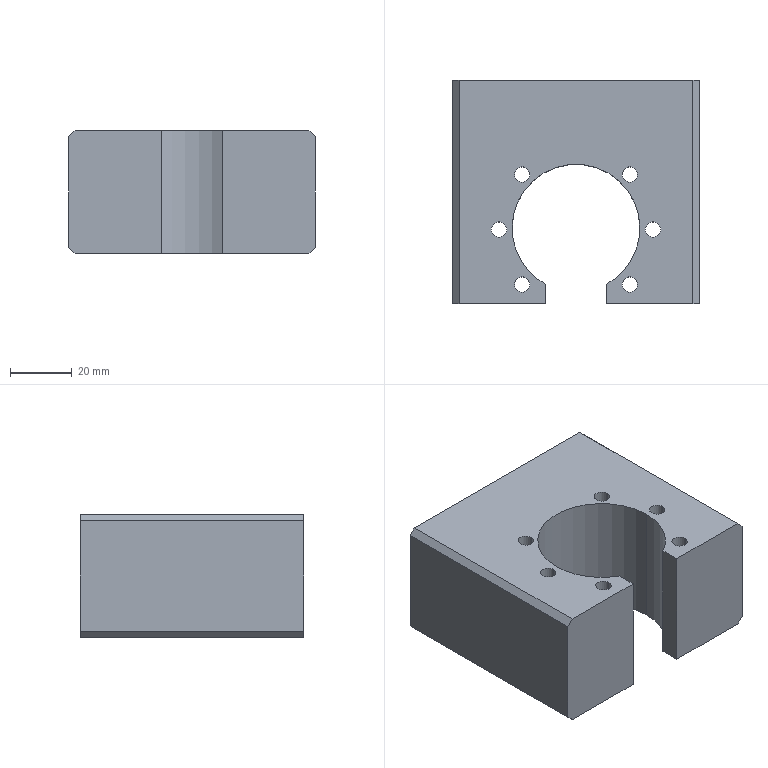Part | SolidWorks | features HoleWzd 2, Chamfer 1, Extrusion 1, ICE 1 | 1 solid | 52 faces | box 80 x 72.5 x 40 mm | volume 167108 mm3 | cylinder 27 | plane 13 | cone 12 | commonest cylinder face diameters 5 x24 41.5 x3
STEP:
#1=CARTESIAN_POINT('',(-27.5,21.25,-13.5));
#2=VERTEX_POINT('',#1);
#3=CARTESIAN_POINT('',(-27.5,21.25,-8.5));
#4=VERTEX_POINT('',#3);
#5=CARTESIAN_POINT('',(-27.5,21.25,-11.));
#6=DIRECTION('',(0.,1.,0.));
#7=DIRECTION('',(0.,0.,1.));
#8=AXIS2_PLACEMENT_3D('',#5,#6,#7);
#9=CIRCLE('',#8,2.5);
#10=EDGE_CURVE('',#2,#4,#9,.T.);
#11=ORIENTED_EDGE('',*,*,#10,.F.);
#12=CARTESIAN_POINT('',(-27.5,36.25,-13.5));
#13=VERTEX_POINT('',#12);
#14=CARTESIAN_POINT('',(-27.5,36.25,-13.5));
#15=DIRECTION('',(0.,1.,0.));
#16=VECTOR('',#15,1000.);
#17=LINE('',#14,#16);
#18=EDGE_CURVE('',#2,#13,#17,.T.);
#19=ORIENTED_EDGE('',*,*,#18,.T.);
#20=CARTESIAN_POINT('',(-27.5,36.25,-8.5));
#21=VERTEX_POINT('',#20);
#22=CARTESIAN_POINT('',(-27.5,36.25,-11.));
#23=DIRECTION('',(0.,1.,0.));
#24=DIRECTION('',(0.,0.,1.));
#25=AXIS2_PLACEMENT_3D('',#22,#23,#24);
#26=CIRCLE('',#25,2.5);
#27=EDGE_CURVE('',#13,#21,#26,.T.);
#28=ORIENTED_EDGE('',*,*,#27,.T.);
#29=CARTESIAN_POINT('',(-27.5,36.25,-8.5));
#30=DIRECTION('',(0.,1.,0.));
#31=VECTOR('',#30,1000.);
#32=LINE('',#29,#31);
#33=EDGE_CURVE('',#4,#21,#32,.T.);
#34=ORIENTED_EDGE('',*,*,#33,.F.);
#35=EDGE_LOOP('',(#11,#19,#28,#34));
#36=FACE_OUTER_BOUND('',#35,.T.);
#37=CARTESIAN_POINT('',(-27.5,36.25,-11.));
#38=DIRECTION('',(0.,1.,0.));
#39=DIRECTION('',(0.,0.,1.));
#40=AXIS2_PLACEMENT_3D('',#37,#38,#39);
#41=CYLINDRICAL_SURFACE('',#40,2.5);
#42=ADVANCED_FACE('',(#36),#41,.F.);
#43=CARTESIAN_POINT('',(-27.5,19.748,-11.));
#44=VERTEX_POINT('',#43);
#45=CARTESIAN_POINT('',(-27.5,21.25,-8.5));
#46=DIRECTION('',(0.,0.515,0.8572));
#47=VECTOR('',#46,1000.);
#48=LINE('',#45,#47);
#49=EDGE_CURVE('',#44,#4,#48,.T.);
#50=ORIENTED_EDGE('',*,*,#49,.F.);
#51=CARTESIAN_POINT('',(-27.5,21.25,-13.5));
#52=DIRECTION('',(0.,0.515,-0.8572));
#53=VECTOR('',#52,1000.);
#54=LINE('',#51,#53);
#55=EDGE_CURVE('',#44,#2,#54,.T.);
#56=ORIENTED_EDGE('',*,*,#55,.T.);
#57=ORIENTED_EDGE('',*,*,#10,.T.);
#58=EDGE_LOOP('',(#50,#56,#57));
#59=FACE_OUTER_BOUND('',#58,.T.);
#60=CARTESIAN_POINT('',(-27.5,21.25,-11.));
#61=DIRECTION('',(0.,1.,0.));
#62=DIRECTION('',(0.,0.,1.));
#63=AXIS2_PLACEMENT_3D('',#60,#61,#62);
#64=CONICAL_SURFACE('',#63,2.5,1.03);
#65=ADVANCED_FACE('',(#59),#64,.F.);
#66=CARTESIAN_POINT('',(-27.5,21.25,8.5));
#67=VERTEX_POINT('',#66);
#68=CARTESIAN_POINT('',(-27.5,21.25,13.5));
#69=VERTEX_POINT('',#68);
#70=CARTESIAN_POINT('',(-27.5,21.25,11.));
#71=DIRECTION('',(0.,1.,0.));
#72=DIRECTION('',(0.,0.,1.));
#73=AXIS2_PLACEMENT_3D('',#70,#71,#72);
#74=CIRCLE('',#73,2.5);
#75=EDGE_CURVE('',#67,#69,#74,.T.);
#76=ORIENTED_EDGE('',*,*,#75,.F.);
#77=CARTESIAN_POINT('',(-27.5,36.25,8.5));
#78=VERTEX_POINT('',#77);
#79=CARTESIAN_POINT('',(-27.5,36.25,8.5));
#80=DIRECTION('',(0.,1.,0.));
#81=VECTOR('',#80,1000.);
#82=LINE('',#79,#81);
#83=EDGE_CURVE('',#67,#78,#82,.T.);
#84=ORIENTED_EDGE('',*,*,#83,.T.);
#85=CARTESIAN_POINT('',(-27.5,36.25,13.5));
#86=VERTEX_POINT('',#85);
#87=CARTESIAN_POINT('',(-27.5,36.25,11.));
#88=DIRECTION('',(0.,1.,0.));
#89=DIRECTION('',(0.,0.,1.));
#90=AXIS2_PLACEMENT_3D('',#87,#88,#89);
#91=CIRCLE('',#90,2.5);
#92=EDGE_CURVE('',#78,#86,#91,.T.);
#93=ORIENTED_EDGE('',*,*,#92,.T.);
#94=CARTESIAN_POINT('',(-27.5,36.25,13.5));
#95=DIRECTION('',(0.,1.,0.));
#96=VECTOR('',#95,1000.);
#97=LINE('',#94,#96);
#98=EDGE_CURVE('',#69,#86,#97,.T.);
#99=ORIENTED_EDGE('',*,*,#98,.F.);
#100=EDGE_LOOP('',(#76,#84,#93,#99));
#101=FACE_OUTER_BOUND('',#100,.T.);
#102=CARTESIAN_POINT('',(-27.5,36.25,11.));
#103=DIRECTION('',(0.,1.,0.));
#104=DIRECTION('',(0.,0.,1.));
#105=AXIS2_PLACEMENT_3D('',#102,#103,#104);
#106=CYLINDRICAL_SURFACE('',#105,2.5);
#107=ADVANCED_FACE('',(#101),#106,.F.);
#108=CARTESIAN_POINT('',(-27.5,19.748,11.));
#109=VERTEX_POINT('',#108);
#110=CARTESIAN_POINT('',(-27.5,21.25,13.5));
#111=DIRECTION('',(0.,0.515,0.8572));
#112=VECTOR('',#111,1000.);
#113=LINE('',#110,#112);
#114=EDGE_CURVE('',#109,#69,#113,.T.);
#115=ORIENTED_EDGE('',*,*,#114,.F.);
#116=CARTESIAN_POINT('',(-27.5,21.25,8.5));
#117=DIRECTION('',(0.,0.515,-0.8572));
#118=VECTOR('',#117,1000.);
#119=LINE('',#116,#118);
#120=EDGE_CURVE('',#109,#67,#119,.T.);
#121=ORIENTED_EDGE('',*,*,#120,.T.);
#122=ORIENTED_EDGE('',*,*,#75,.T.);
#123=EDGE_LOOP('',(#115,#121,#122));
#124=FACE_OUTER_BOUND('',#123,.T.);
#125=CARTESIAN_POINT('',(-27.5,21.25,11.));
#126=DIRECTION('',(0.,1.,0.));
#127=DIRECTION('',(0.,0.,1.));
#128=AXIS2_PLACEMENT_3D('',#125,#126,#127);
#129=CONICAL_SURFACE('',#128,2.5,1.03);
#130=ADVANCED_FACE('',(#124),#129,.F.);
#131=CARTESIAN_POINT('',(27.5,21.25,8.5));
#132=VERTEX_POINT('',#131);
#133=CARTESIAN_POINT('',(27.5,21.25,13.5));
#134=VERTEX_POINT('',#133);
#135=CARTESIAN_POINT('',(27.5,21.25,11.));
#136=DIRECTION('',(0.,1.,0.));
#137=DIRECTION('',(0.,0.,1.));
#138=AXIS2_PLACEMENT_3D('',#135,#136,#137);
#139=CIRCLE('',#138,2.5);
#140=EDGE_CURVE('',#132,#134,#139,.T.);
#141=ORIENTED_EDGE('',*,*,#140,.F.);
#142=CARTESIAN_POINT('',(27.5,36.25,8.5));
#143=VERTEX_POINT('',#142);
#144=CARTESIAN_POINT('',(27.5,36.25,8.5));
#145=DIRECTION('',(0.,1.,0.));
#146=VECTOR('',#145,1000.);
#147=LINE('',#144,#146);
#148=EDGE_CURVE('',#132,#143,#147,.T.);
#149=ORIENTED_EDGE('',*,*,#148,.T.);
#150=CARTESIAN_POINT('',(27.5,36.25,13.5));
#151=VERTEX_POINT('',#150);
#152=CARTESIAN_POINT('',(27.5,36.25,11.));
#153=DIRECTION('',(0.,1.,0.));
#154=DIRECTION('',(0.,0.,1.));
#155=AXIS2_PLACEMENT_3D('',#152,#153,#154);
#156=CIRCLE('',#155,2.5);
#157=EDGE_CURVE('',#143,#151,#156,.T.);
#158=ORIENTED_EDGE('',*,*,#157,.T.);
#159=CARTESIAN_POINT('',(27.5,36.25,13.5));
#160=DIRECTION('',(0.,1.,0.));
#161=VECTOR('',#160,1000.);
#162=LINE('',#159,#161);
#163=EDGE_CURVE('',#134,#151,#162,.T.);
#164=ORIENTED_EDGE('',*,*,#163,.F.);
#165=EDGE_LOOP('',(#141,#149,#158,#164));
#166=FACE_OUTER_BOUND('',#165,.T.);
#167=CARTESIAN_POINT('',(27.5,36.25,11.));
#168=DIRECTION('',(0.,1.,0.));
#169=DIRECTION('',(0.,0.,1.));
#170=AXIS2_PLACEMENT_3D('',#167,#168,#169);
#171=CYLINDRICAL_SURFACE('',#170,2.5);
#172=ADVANCED_FACE('',(#166),#171,.F.);
#173=CARTESIAN_POINT('',(27.5,19.748,11.));
#174=VERTEX_POINT('',#173);
#175=CARTESIAN_POINT('',(27.5,21.25,13.5));
#176=DIRECTION('',(0.,0.515,0.8572));
#177=VECTOR('',#176,1000.);
#178=LINE('',#175,#177);
#179=EDGE_CURVE('',#174,#134,#178,.T.);
#180=ORIENTED_EDGE('',*,*,#179,.F.);
#181=CARTESIAN_POINT('',(27.5,21.25,8.5));
#182=DIRECTION('',(0.,0.515,-0.8572));
#183=VECTOR('',#182,1000.);
#184=LINE('',#181,#183);
#185=EDGE_CURVE('',#174,#132,#184,.T.);
#186=ORIENTED_EDGE('',*,*,#185,.T.);
#187=ORIENTED_EDGE('',*,*,#140,.T.);
#188=EDGE_LOOP('',(#180,#186,#187));
#189=FACE_OUTER_BOUND('',#188,.T.);
#190=CARTESIAN_POINT('',(27.5,21.25,11.));
#191=DIRECTION('',(0.,1.,0.));
#192=DIRECTION('',(0.,0.,1.));
#193=AXIS2_PLACEMENT_3D('',#190,#191,#192);
#194=CONICAL_SURFACE('',#193,2.5,1.03);
#195=ADVANCED_FACE('',(#189),#194,.F.);
#196=CARTESIAN_POINT('',(27.5,21.25,-13.5));
#197=VERTEX_POINT('',#196);
#198=CARTESIAN_POINT('',(27.5,21.25,-8.5));
#199=VERTEX_POINT('',#198);
#200=CARTESIAN_POINT('',(27.5,21.25,-11.));
#201=DIRECTION('',(0.,1.,0.));
#202=DIRECTION('',(0.,0.,1.));
#203=AXIS2_PLACEMENT_3D('',#200,#201,#202);
#204=CIRCLE('',#203,2.5);
#205=EDGE_CURVE('',#197,#199,#204,.T.);
#206=ORIENTED_EDGE('',*,*,#205,.F.);
#207=CARTESIAN_POINT('',(27.5,36.25,-13.5));
#208=VERTEX_POINT('',#207);
#209=CARTESIAN_POINT('',(27.5,36.25,-13.5));
#210=DIRECTION('',(0.,1.,0.));
#211=VECTOR('',#210,1000.);
#212=LINE('',#209,#211);
#213=EDGE_CURVE('',#197,#208,#212,.T.);
#214=ORIENTED_EDGE('',*,*,#213,.T.);
#215=CARTESIAN_POINT('',(27.5,36.25,-8.5));
#216=VERTEX_POINT('',#215);
#217=CARTESIAN_POINT('',(27.5,36.25,-11.));
#218=DIRECTION('',(0.,1.,0.));
#219=DIRECTION('',(0.,0.,1.));
#220=AXIS2_PLACEMENT_3D('',#217,#218,#219);
#221=CIRCLE('',#220,2.5);
#222=EDGE_CURVE('',#208,#216,#221,.T.);
#223=ORIENTED_EDGE('',*,*,#222,.T.);
#224=CARTESIAN_POINT('',(27.5,36.25,-8.5));
#225=DIRECTION('',(0.,1.,0.));
#226=VECTOR('',#225,1000.);
#227=LINE('',#224,#226);
#228=EDGE_CURVE('',#199,#216,#227,.T.);
#229=ORIENTED_EDGE('',*,*,#228,.F.);
#230=EDGE_LOOP('',(#206,#214,#223,#229));
#231=FACE_OUTER_BOUND('',#230,.T.);
#232=CARTESIAN_POINT('',(27.5,36.25,-11.));
#233=DIRECTION('',(0.,1.,0.));
#234=DIRECTION('',(0.,0.,1.));
#235=AXIS2_PLACEMENT_3D('',#232,#233,#234);
#236=CYLINDRICAL_SURFACE('',#235,2.5);
#237=ADVANCED_FACE('',(#231),#236,.F.);
#238=CARTESIAN_POINT('',(27.5,19.748,-11.));
#239=VERTEX_POINT('',#238);
#240=CARTESIAN_POINT('',(27.5,21.25,-8.5));
#241=DIRECTION('',(0.,0.515,0.8572));
#242=VECTOR('',#241,1000.);
#243=LINE('',#240,#242);
#244=EDGE_CURVE('',#239,#199,#243,.T.);
#245=ORIENTED_EDGE('',*,*,#244,.F.);
#246=CARTESIAN_POINT('',(27.5,21.25,-13.5));
#247=DIRECTION('',(0.,0.515,-0.8572));
#248=VECTOR('',#247,1000.);
#249=LINE('',#246,#248);
#250=EDGE_CURVE('',#239,#197,#249,.T.);
#251=ORIENTED_EDGE('',*,*,#250,.T.);
#252=ORIENTED_EDGE('',*,*,#205,.T.);
#253=EDGE_LOOP('',(#245,#251,#252));
#254=FACE_OUTER_BOUND('',#253,.T.);
#255=CARTESIAN_POINT('',(27.5,21.25,-11.));
#256=DIRECTION('',(0.,1.,0.));
#257=DIRECTION('',(0.,0.,1.));
#258=AXIS2_PLACEMENT_3D('',#255,#256,#257);
#259=CONICAL_SURFACE('',#258,2.5,1.03);
#260=ADVANCED_FACE('',(#254),#259,.F.);
#261=CARTESIAN_POINT('',(0.,21.25,-13.5));
#262=VERTEX_POINT('',#261);
#263=CARTESIAN_POINT('',(0.,21.25,-8.5));
#264=VERTEX_POINT('',#263);
#265=CARTESIAN_POINT('',(0.,21.25,-11.));
#266=DIRECTION('',(0.,1.,0.));
#267=DIRECTION('',(0.,0.,1.));
#268=AXIS2_PLACEMENT_3D('',#265,#266,#267);
#269=CIRCLE('',#268,2.5);
#270=EDGE_CURVE('',#262,#264,#269,.T.);
#271=ORIENTED_EDGE('',*,*,#270,.F.);
#272=CARTESIAN_POINT('',(0.,36.25,-13.5));
#273=VERTEX_POINT('',#272);
#274=CARTESIAN_POINT('',(0.,36.25,-13.5));
#275=DIRECTION('',(0.,1.,0.));
#276=VECTOR('',#275,1000.);
#277=LINE('',#274,#276);
#278=EDGE_CURVE('',#262,#273,#277,.T.);
#279=ORIENTED_EDGE('',*,*,#278,.T.);
#280=CARTESIAN_POINT('',(0.,36.25,-8.5));
#281=VERTEX_POINT('',#280);
#282=CARTESIAN_POINT('',(0.,36.25,-11.));
#283=DIRECTION('',(0.,1.,0.));
#284=DIRECTION('',(0.,0.,1.));
#285=AXIS2_PLACEMENT_3D('',#282,#283,#284);
#286=CIRCLE('',#285,2.5);
#287=EDGE_CURVE('',#273,#281,#286,.T.);
#288=ORIENTED_EDGE('',*,*,#287,.T.);
#289=CARTESIAN_POINT('',(0.,36.25,-8.5));
#290=DIRECTION('',(0.,1.,0.));
#291=VECTOR('',#290,1000.);
#292=LINE('',#289,#291);
#293=EDGE_CURVE('',#264,#281,#292,.T.);
#294=ORIENTED_EDGE('',*,*,#293,.F.);
#295=EDGE_LOOP('',(#271,#279,#288,#294));
#296=FACE_OUTER_BOUND('',#295,.T.);
#297=CARTESIAN_POINT('',(0.,36.25,-11.));
#298=DIRECTION('',(0.,1.,0.));
#299=DIRECTION('',(0.,0.,1.));
#300=AXIS2_PLACEMENT_3D('',#297,#298,#299);
#301=CYLINDRICAL_SURFACE('',#300,2.5);
#302=ADVANCED_FACE('',(#296),#301,.F.);
#303=CARTESIAN_POINT('',(0.,19.748,-11.));
#304=VERTEX_POINT('',#303);
#305=CARTESIAN_POINT('',(0.,21.25,-8.5));
#306=DIRECTION('',(0.,0.515,0.8572));
#307=VECTOR('',#306,1000.);
#308=LINE('',#305,#307);
#309=EDGE_CURVE('',#304,#264,#308,.T.);
#310=ORIENTED_EDGE('',*,*,#309,.F.);
#311=CARTESIAN_POINT('',(0.,21.25,-13.5));
#312=DIRECTION('',(0.,0.515,-0.8572));
#313=VECTOR('',#312,1000.);
#314=LINE('',#311,#313);
#315=EDGE_CURVE('',#304,#262,#314,.T.);
#316=ORIENTED_EDGE('',*,*,#315,.T.);
#317=ORIENTED_EDGE('',*,*,#270,.T.);
#318=EDGE_LOOP('',(#310,#316,#317));
#319=FACE_OUTER_BOUND('',#318,.T.);
#320=CARTESIAN_POINT('',(0.,21.25,-11.));
#321=DIRECTION('',(0.,1.,0.));
#322=DIRECTION('',(0.,0.,1.));
#323=AXIS2_PLACEMENT_3D('',#320,#321,#322);
#324=CONICAL_SURFACE('',#323,2.5,1.03);
#325=ADVANCED_FACE('',(#319),#324,.F.);
#326=CARTESIAN_POINT('',(0.,21.25,8.5));
#327=VERTEX_POINT('',#326);
#328=CARTESIAN_POINT('',(0.,21.25,13.5));
#329=VERTEX_POINT('',#328);
#330=CARTESIAN_POINT('',(0.,21.25,11.));
#331=DIRECTION('',(0.,1.,0.));
#332=DIRECTION('',(0.,0.,1.));
#333=AXIS2_PLACEMENT_3D('',#330,#331,#332);
#334=CIRCLE('',#333,2.5);
#335=EDGE_CURVE('',#327,#329,#334,.T.);
#336=ORIENTED_EDGE('',*,*,#335,.F.);
#337=CARTESIAN_POINT('',(0.,36.25,8.5));
#338=VERTEX_POINT('',#337);
#339=CARTESIAN_POINT('',(0.,36.25,8.5));
#340=DIRECTION('',(0.,1.,0.));
#341=VECTOR('',#340,1000.);
#342=LINE('',#339,#341);
#343=EDGE_CURVE('',#327,#338,#342,.T.);
#344=ORIENTED_EDGE('',*,*,#343,.T.);
#345=CARTESIAN_POINT('',(0.,36.25,13.5));
#346=VERTEX_POINT('',#345);
#347=CARTESIAN_POINT('',(0.,36.25,11.));
#348=DIRECTION('',(0.,1.,0.));
#349=DIRECTION('',(0.,0.,1.));
#350=AXIS2_PLACEMENT_3D('',#347,#348,#349);
#351=CIRCLE('',#350,2.5);
#352=EDGE_CURVE('',#338,#346,#351,.T.);
#353=ORIENTED_EDGE('',*,*,#352,.T.);
#354=CARTESIAN_POINT('',(0.,36.25,13.5));
#355=DIRECTION('',(0.,1.,0.));
#356=VECTOR('',#355,1000.);
#357=LINE('',#354,#356);
#358=EDGE_CURVE('',#329,#346,#357,.T.);
#359=ORIENTED_EDGE('',*,*,#358,.F.);
#360=EDGE_LOOP('',(#336,#344,#353,#359));
#361=FACE_OUTER_BOUND('',#360,.T.);
#362=CARTESIAN_POINT('',(0.,36.25,11.));
#363=DIRECTION('',(0.,1.,0.));
#364=DIRECTION('',(0.,0.,1.));
#365=AXIS2_PLACEMENT_3D('',#362,#363,#364);
#366=CYLINDRICAL_SURFACE('',#365,2.5);
#367=ADVANCED_FACE('',(#361),#366,.F.);
#368=CARTESIAN_POINT('',(0.,19.748,11.));
#369=VERTEX_POINT('',#368);
#370=CARTESIAN_POINT('',(0.,21.25,13.5));
#371=DIRECTION('',(0.,0.515,0.8572));
#372=VECTOR('',#371,1000.);
#373=LINE('',#370,#372);
#374=EDGE_CURVE('',#369,#329,#373,.T.);
#375=ORIENTED_EDGE('',*,*,#374,.F.);
#376=CARTESIAN_POINT('',(0.,21.25,8.5));
#377=DIRECTION('',(0.,0.515,-0.8572));
#378=VECTOR('',#377,1000.);
#379=LINE('',#376,#378);
#380=EDGE_CURVE('',#369,#327,#379,.T.);
#381=ORIENTED_EDGE('',*,*,#380,.T.);
#382=ORIENTED_EDGE('',*,*,#335,.T.);
#383=EDGE_LOOP('',(#375,#381,#382));
#384=FACE_OUTER_BOUND('',#383,.T.);
#385=CARTESIAN_POINT('',(0.,21.25,11.));
#386=DIRECTION('',(0.,1.,0.));
#387=DIRECTION('',(0.,0.,1.));
#388=AXIS2_PLACEMENT_3D('',#385,#386,#387);
#389=CONICAL_SURFACE('',#388,2.5,1.03);
#390=ADVANCED_FACE('',(#384),#389,.F.);
#391=CARTESIAN_POINT('',(20.,5.604,20.));
#392=VERTEX_POINT('',#391);
#393=CARTESIAN_POINT('',(15.,5.604,20.));
#394=VERTEX_POINT('',#393);
#395=CARTESIAN_POINT('',(17.5,5.604,20.));
#396=DIRECTION('',(0.,0.,-1.));
#397=DIRECTION('',(-1.,0.,0.));
#398=AXIS2_PLACEMENT_3D('',#395,#396,#397);
#399=CIRCLE('',#398,2.5);
#400=EDGE_CURVE('',#392,#394,#399,.T.);
#401=ORIENTED_EDGE('',*,*,#400,.F.);
#402=CARTESIAN_POINT('',(20.,5.604,-20.));
#403=VERTEX_POINT('',#402);
#404=CARTESIAN_POINT('',(20.,5.604,-20.));
#405=DIRECTION('',(0.,0.,-1.));
#406=VECTOR('',#405,1000.);
#407=LINE('',#404,#406);
#408=EDGE_CURVE('',#392,#403,#407,.T.);
#409=ORIENTED_EDGE('',*,*,#408,.T.);
#410=CARTESIAN_POINT('',(15.,5.604,-20.));
#411=VERTEX_POINT('',#410);
#412=CARTESIAN_POINT('',(17.5,5.604,-20.));
#413=DIRECTION('',(0.,0.,-1.));
#414=DIRECTION('',(-1.,0.,0.));
#415=AXIS2_PLACEMENT_3D('',#412,#413,#414);
#416=CIRCLE('',#415,2.5);
#417=EDGE_CURVE('',#403,#411,#416,.T.);
#418=ORIENTED_EDGE('',*,*,#417,.T.);
#419=CARTESIAN_POINT('',(15.,5.604,-20.));
#420=DIRECTION('',(0.,0.,-1.));
#421=VECTOR('',#420,1000.);
#422=LINE('',#419,#421);
#423=EDGE_CURVE('',#394,#411,#422,.T.);
#424=ORIENTED_EDGE('',*,*,#423,.F.);
#425=EDGE_LOOP('',(#401,#409,#418,#424));
#426=FACE_OUTER_BOUND('',#425,.T.);
#427=CARTESIAN_POINT('',(17.5,5.604,-20.));
#428=DIRECTION('',(0.,0.,-1.));
#429=DIRECTION('',(-1.,0.,0.));
#430=AXIS2_PLACEMENT_3D('',#427,#428,#429);
#431=CYLINDRICAL_SURFACE('',#430,2.5);
#432=ADVANCED_FACE('',(#426),#431,.F.);
#433=CARTESIAN_POINT('',(-15.,5.604,20.));
#434=VERTEX_POINT('',#433);
#435=CARTESIAN_POINT('',(-20.,5.604,20.));
#436=VERTEX_POINT('',#435);
#437=CARTESIAN_POINT('',(-17.5,5.604,20.));
#438=DIRECTION('',(0.,0.,-1.));
#439=DIRECTION('',(-1.,0.,0.));
#440=AXIS2_PLACEMENT_3D('',#437,#438,#439);
#441=CIRCLE('',#440,2.5);
#442=EDGE_CURVE('',#434,#436,#441,.T.);
#443=ORIENTED_EDGE('',*,*,#442,.F.);
#444=CARTESIAN_POINT('',(-15.,5.604,-20.));
#445=VERTEX_POINT('',#444);
#446=CARTESIAN_POINT('',(-15.,5.604,-20.));
#447=DIRECTION('',(0.,0.,-1.));
#448=VECTOR('',#447,1000.);
#449=LINE('',#446,#448);
#450=EDGE_CURVE('',#434,#445,#449,.T.);
#451=ORIENTED_EDGE('',*,*,#450,.T.);
#452=CARTESIAN_POINT('',(-20.,5.604,-20.));
#453=VERTEX_POINT('',#452);
#454=CARTESIAN_POINT('',(-17.5,5.604,-20.));
#455=DIRECTION('',(0.,0.,-1.));
#456=DIRECTION('',(-1.,0.,0.));
#457=AXIS2_PLACEMENT_3D('',#454,#455,#456);
#458=CIRCLE('',#457,2.5);
#459=EDGE_CURVE('',#445,#453,#458,.T.);
#460=ORIENTED_EDGE('',*,*,#459,.T.);
#461=CARTESIAN_POINT('',(-20.,5.604,-20.));
#462=DIRECTION('',(0.,0.,-1.));
#463=VECTOR('',#462,1000.);
#464=LINE('',#461,#463);
#465=EDGE_CURVE('',#436,#453,#464,.T.);
#466=ORIENTED_EDGE('',*,*,#465,.F.);
#467=EDGE_LOOP('',(#443,#451,#460,#466));
#468=FACE_OUTER_BOUND('',#467,.T.);
#469=CARTESIAN_POINT('',(-17.5,5.604,-20.));
#470=DIRECTION('',(0.,0.,-1.));
#471=DIRECTION('',(-1.,0.,0.));
#472=AXIS2_PLACEMENT_3D('',#469,#470,#471);
#473=CYLINDRICAL_SURFACE('',#472,2.5);
#474=ADVANCED_FACE('',(#468),#473,.F.);
#475=CARTESIAN_POINT('',(-15.,-30.104,20.));
#476=VERTEX_POINT('',#475);
#477=CARTESIAN_POINT('',(-20.,-30.104,20.));
#478=VERTEX_POINT('',#477);
#479=CARTESIAN_POINT('',(-17.5,-30.104,20.));
#480=DIRECTION('',(0.,0.,-1.));
#481=DIRECTION('',(-1.,0.,0.));
#482=AXIS2_PLACEMENT_3D('',#479,#480,#481);
#483=CIRCLE('',#482,2.5);
#484=EDGE_CURVE('',#476,#478,#483,.T.);
#485=ORIENTED_EDGE('',*,*,#484,.F.);
#486=CARTESIAN_POINT('',(-15.,-30.104,-20.));
#487=VERTEX_POINT('',#486);
#488=CARTESIAN_POINT('',(-15.,-30.104,-20.));
#489=DIRECTION('',(0.,0.,-1.));
#490=VECTOR('',#489,1000.);
#491=LINE('',#488,#490);
#492=EDGE_CURVE('',#476,#487,#491,.T.);
#493=ORIENTED_EDGE('',*,*,#492,.T.);
#494=CARTESIAN_POINT('',(-20.,-30.104,-20.));
#495=VERTEX_POINT('',#494);
#496=CARTESIAN_POINT('',(-17.5,-30.104,-20.));
#497=DIRECTION('',(0.,0.,-1.));
#498=DIRECTION('',(-1.,0.,0.));
#499=AXIS2_PLACEMENT_3D('',#496,#497,#498);
#500=CIRCLE('',#499,2.5);
#501=EDGE_CURVE('',#487,#495,#500,.T.);
#502=ORIENTED_EDGE('',*,*,#501,.T.);
#503=CARTESIAN_POINT('',(-20.,-30.104,-20.));
#504=DIRECTION('',(0.,0.,-1.));
#505=VECTOR('',#504,1000.);
#506=LINE('',#503,#505);
#507=EDGE_CURVE('',#478,#495,#506,.T.);
#508=ORIENTED_EDGE('',*,*,#507,.F.);
#509=EDGE_LOOP('',(#485,#493,#502,#508));
#510=FACE_OUTER_BOUND('',#509,.T.);
#511=CARTESIAN_POINT('',(-17.5,-30.104,-20.));
#512=DIRECTION('',(0.,0.,-1.));
#513=DIRECTION('',(-1.,0.,0.));
#514=AXIS2_PLACEMENT_3D('',#511,#512,#513);
#515=CYLINDRICAL_SURFACE('',#514,2.5);
#516=ADVANCED_FACE('',(#510),#515,.F.);
#517=CARTESIAN_POINT('',(20.,-30.104,20.));
#518=VERTEX_POINT('',#517);
#519=CARTESIAN_POINT('',(15.,-30.104,20.));
#520=VERTEX_POINT('',#519);
#521=CARTESIAN_POINT('',(17.5,-30.104,20.));
#522=DIRECTION('',(0.,0.,-1.));
#523=DIRECTION('',(-1.,0.,0.));
#524=AXIS2_PLACEMENT_3D('',#521,#522,#523);
#525=CIRCLE('',#524,2.5);
#526=EDGE_CURVE('',#518,#520,#525,.T.);
#527=ORIENTED_EDGE('',*,*,#526,.F.);
#528=CARTESIAN_POINT('',(20.,-30.104,-20.));
#529=VERTEX_POINT('',#528);
#530=CARTESIAN_POINT('',(20.,-30.104,-20.));
#531=DIRECTION('',(0.,0.,-1.));
#532=VECTOR('',#531,1000.);
#533=LINE('',#530,#532);
#534=EDGE_CURVE('',#518,#529,#533,.T.);
#535=ORIENTED_EDGE('',*,*,#534,.T.);
#536=CARTESIAN_POINT('',(15.,-30.104,-20.));
#537=VERTEX_POINT('',#536);
#538=CARTESIAN_POINT('',(17.5,-30.104,-20.));
#539=DIRECTION('',(0.,0.,-1.));
#540=DIRECTION('',(-1.,0.,0.));
#541=AXIS2_PLACEMENT_3D('',#538,#539,#540);
#542=CIRCLE('',#541,2.5);
#543=EDGE_CURVE('',#529,#537,#542,.T.);
#544=ORIENTED_EDGE('',*,*,#543,.T.);
#545=CARTESIAN_POINT('',(15.,-30.104,-20.));
#546=DIRECTION('',(0.,0.,-1.));
#547=VECTOR('',#546,1000.);
#548=LINE('',#545,#547);
#549=EDGE_CURVE('',#520,#537,#548,.T.);
#550=ORIENTED_EDGE('',*,*,#549,.F.);
#551=EDGE_LOOP('',(#527,#535,#544,#550));
#552=FACE_OUTER_BOUND('',#551,.T.);
#553=CARTESIAN_POINT('',(17.5,-30.104,-20.));
#554=DIRECTION('',(0.,0.,-1.));
#555=DIRECTION('',(-1.,0.,0.));
#556=AXIS2_PLACEMENT_3D('',#553,#554,#555);
#557=CYLINDRICAL_SURFACE('',#556,2.5);
#558=ADVANCED_FACE('',(#552),#557,.F.);
#559=CARTESIAN_POINT('',(27.5,-12.25,20.));
#560=VERTEX_POINT('',#559);
#561=CARTESIAN_POINT('',(22.5,-12.25,20.));
#562=VERTEX_POINT('',#561);
#563=CARTESIAN_POINT('',(25.,-12.25,20.));
#564=DIRECTION('',(0.,0.,-1.));
#565=DIRECTION('',(-1.,0.,0.));
#566=AXIS2_PLACEMENT_3D('',#563,#564,#565);
#567=CIRCLE('',#566,2.5);
#568=EDGE_CURVE('',#560,#562,#567,.T.);
#569=ORIENTED_EDGE('',*,*,#568,.F.);
#570=CARTESIAN_POINT('',(27.5,-12.25,-20.));
#571=VERTEX_POINT('',#570);
#572=CARTESIAN_POINT('',(27.5,-12.25,-20.));
#573=DIRECTION('',(0.,0.,-1.));
#574=VECTOR('',#573,1000.);
#575=LINE('',#572,#574);
#576=EDGE_CURVE('',#560,#571,#575,.T.);
#577=ORIENTED_EDGE('',*,*,#576,.T.);
#578=CARTESIAN_POINT('',(22.5,-12.25,-20.));
#579=VERTEX_POINT('',#578);
#580=CARTESIAN_POINT('',(25.,-12.25,-20.));
#581=DIRECTION('',(0.,0.,-1.));
#582=DIRECTION('',(-1.,0.,0.));
#583=AXIS2_PLACEMENT_3D('',#580,#581,#582);
#584=CIRCLE('',#583,2.5);
#585=EDGE_CURVE('',#571,#579,#584,.T.);
#586=ORIENTED_EDGE('',*,*,#585,.T.);
#587=CARTESIAN_POINT('',(22.5,-12.25,-20.));
#588=DIRECTION('',(0.,0.,-1.));
#589=VECTOR('',#588,1000.);
#590=LINE('',#587,#589);
#591=EDGE_CURVE('',#562,#579,#590,.T.);
#592=ORIENTED_EDGE('',*,*,#591,.F.);
#593=EDGE_LOOP('',(#569,#577,#586,#592));
#594=FACE_OUTER_BOUND('',#593,.T.);
#595=CARTESIAN_POINT('',(25.,-12.25,-20.));
#596=DIRECTION('',(0.,0.,-1.));
#597=DIRECTION('',(-1.,0.,0.));
#598=AXIS2_PLACEMENT_3D('',#595,#596,#597);
#599=CYLINDRICAL_SURFACE('',#598,2.5);
#600=ADVANCED_FACE('',(#594),#599,.F.);
#601=CARTESIAN_POINT('',(-22.5,-12.25,20.));
#602=VERTEX_POINT('',#601);
#603=CARTESIAN_POINT('',(-27.5,-12.25,20.));
#604=VERTEX_POINT('',#603);
#605=CARTESIAN_POINT('',(-25.,-12.25,20.));
#606=DIRECTION('',(0.,0.,-1.));
#607=DIRECTION('',(-1.,0.,0.));
#608=AXIS2_PLACEMENT_3D('',#605,#606,#607);
#609=CIRCLE('',#608,2.5);
#610=EDGE_CURVE('',#602,#604,#609,.T.);
#611=ORIENTED_EDGE('',*,*,#610,.F.);
#612=CARTESIAN_POINT('',(-22.5,-12.25,-20.));
#613=VERTEX_POINT('',#612);
#614=CARTESIAN_POINT('',(-22.5,-12.25,-20.));
#615=DIRECTION('',(0.,0.,-1.));
#616=VECTOR('',#615,1000.);
#617=LINE('',#614,#616);
#618=EDGE_CURVE('',#602,#613,#617,.T.);
#619=ORIENTED_EDGE('',*,*,#618,.T.);
#620=CARTESIAN_POINT('',(-27.5,-12.25,-20.));
#621=VERTEX_POINT('',#620);
#622=CARTESIAN_POINT('',(-25.,-12.25,-20.));
#623=DIRECTION('',(0.,0.,-1.));
#624=DIRECTION('',(-1.,0.,0.));
#625=AXIS2_PLACEMENT_3D('',#622,#623,#624);
#626=CIRCLE('',#625,2.5);
#627=EDGE_CURVE('',#613,#621,#626,.T.);
#628=ORIENTED_EDGE('',*,*,#627,.T.);
#629=CARTESIAN_POINT('',(-27.5,-12.25,-20.));
#630=DIRECTION('',(0.,0.,-1.));
#631=VECTOR('',#630,1000.);
#632=LINE('',#629,#631);
#633=EDGE_CURVE('',#604,#621,#632,.T.);
#634=ORIENTED_EDGE('',*,*,#633,.F.);
#635=EDGE_LOOP('',(#611,#619,#628,#634));
#636=FACE_OUTER_BOUND('',#635,.T.);
#637=CARTESIAN_POINT('',(-25.,-12.25,-20.));
#638=DIRECTION('',(0.,0.,-1.));
#639=DIRECTION('',(-1.,0.,0.));
#640=AXIS2_PLACEMENT_3D('',#637,#638,#639);
#641=CYLINDRICAL_SURFACE('',#640,2.5);
#642=ADVANCED_FACE('',(#636),#641,.F.);
#643=CARTESIAN_POINT('',(10.,-29.931,20.));
#644=VERTEX_POINT('',#643);
#645=CARTESIAN_POINT('',(20.75,-11.75,20.));
#646=VERTEX_POINT('',#645);
#647=CARTESIAN_POINT('',(0.,-11.75,20.));
#648=DIRECTION('',(0.,0.,1.));
#649=DIRECTION('',(1.,0.,0.));
#650=AXIS2_PLACEMENT_3D('',#647,#648,#649);
#651=CIRCLE('',#650,20.75);
#652=EDGE_CURVE('',#644,#646,#651,.T.);
#653=ORIENTED_EDGE('',*,*,#652,.T.);
#654=CARTESIAN_POINT('',(20.75,-11.75,-20.));
#655=VERTEX_POINT('',#654);
#656=CARTESIAN_POINT('',(20.75,-11.75,20.));
#657=DIRECTION('',(0.,0.,-1.));
#658=VECTOR('',#657,1000.);
#659=LINE('',#656,#658);
#660=EDGE_CURVE('',#646,#655,#659,.T.);
#661=ORIENTED_EDGE('',*,*,#660,.T.);
#662=CARTESIAN_POINT('',(10.,-29.931,-20.));
#663=VERTEX_POINT('',#662);
#664=CARTESIAN_POINT('',(0.,-11.75,-20.));
#665=DIRECTION('',(0.,0.,1.));
#666=DIRECTION('',(1.,0.,0.));
#667=AXIS2_PLACEMENT_3D('',#664,#665,#666);
#668=CIRCLE('',#667,20.75);
#669=EDGE_CURVE('',#663,#655,#668,.T.);
#670=ORIENTED_EDGE('',*,*,#669,.F.);
#671=CARTESIAN_POINT('',(10.,-29.931,-20.));
#672=DIRECTION('',(0.,0.,1.));
#673=VECTOR('',#672,1000.);
#674=LINE('',#671,#673);
#675=EDGE_CURVE('',#663,#644,#674,.T.);
#676=ORIENTED_EDGE('',*,*,#675,.T.);
#677=EDGE_LOOP('',(#653,#661,#670,#676));
#678=FACE_OUTER_BOUND('',#677,.T.);
#679=CARTESIAN_POINT('',(0.,-11.75,20.));
#680=DIRECTION('',(0.,0.,-1.));
#681=DIRECTION('',(-1.,0.,0.));
#682=AXIS2_PLACEMENT_3D('',#679,#680,#681);
#683=CYLINDRICAL_SURFACE('',#682,20.75);
#684=ADVANCED_FACE('',(#678),#683,.F.);
#685=ORIENTED_EDGE('',*,*,#660,.F.);
#686=CARTESIAN_POINT('',(-20.75,-11.75,20.));
#687=VERTEX_POINT('',#686);
#688=CARTESIAN_POINT('',(0.,-11.75,20.));
#689=DIRECTION('',(0.,0.,1.));
#690=DIRECTION('',(1.,0.,0.));
#691=AXIS2_PLACEMENT_3D('',#688,#689,#690);
#692=CIRCLE('',#691,20.75);
#693=EDGE_CURVE('',#646,#687,#692,.T.);
#694=ORIENTED_EDGE('',*,*,#693,.T.);
#695=CARTESIAN_POINT('',(-20.75,-11.75,-20.));
#696=VERTEX_POINT('',#695);
#697=CARTESIAN_POINT('',(-20.75,-11.75,20.));
#698=DIRECTION('',(0.,0.,-1.));
#699=VECTOR('',#698,1000.);
#700=LINE('',#697,#699);
#701=EDGE_CURVE('',#687,#696,#700,.T.);
#702=ORIENTED_EDGE('',*,*,#701,.T.);
#703=CARTESIAN_POINT('',(0.,-11.75,-20.));
#704=DIRECTION('',(0.,0.,1.));
#705=DIRECTION('',(1.,0.,0.));
#706=AXIS2_PLACEMENT_3D('',#703,#704,#705);
#707=CIRCLE('',#706,20.75);
#708=EDGE_CURVE('',#655,#696,#707,.T.);
#709=ORIENTED_EDGE('',*,*,#708,.F.);
#710=EDGE_LOOP('',(#685,#694,#702,#709));
#711=FACE_OUTER_BOUND('',#710,.T.);
#712=CARTESIAN_POINT('',(0.,-11.75,20.));
#713=DIRECTION('',(0.,0.,-1.));
#714=DIRECTION('',(-1.,0.,0.));
#715=AXIS2_PLACEMENT_3D('',#712,#713,#714);
#716=CYLINDRICAL_SURFACE('',#715,20.75);
#717=ADVANCED_FACE('',(#711),#716,.F.);
#718=CARTESIAN_POINT('',(-40.,-36.25,18.));
#719=VERTEX_POINT('',#718);
#720=CARTESIAN_POINT('',(-40.,-36.25,-18.));
#721=VERTEX_POINT('',#720);
#722=CARTESIAN_POINT('',(-40.,-36.25,20.));
#723=DIRECTION('',(0.,0.,-1.));
#724=VECTOR('',#723,1000.);
#725=LINE('',#722,#724);
#726=EDGE_CURVE('',#719,#721,#725,.T.);
#727=ORIENTED_EDGE('',*,*,#726,.T.);
#728=CARTESIAN_POINT('',(-38.,-36.25,-20.));
#729=VERTEX_POINT('',#728);
#730=CARTESIAN_POINT('',(-40.,-36.25,-18.));
#731=DIRECTION('',(0.7071,0.,-0.7071));
#732=VECTOR('',#731,1000.);
#733=LINE('',#730,#732);
#734=EDGE_CURVE('',#721,#729,#733,.T.);
#735=ORIENTED_EDGE('',*,*,#734,.T.);
#736=CARTESIAN_POINT('',(-10.,-36.25,-20.));
#737=VERTEX_POINT('',#736);
#738=CARTESIAN_POINT('',(-40.,-36.25,-20.));
#739=DIRECTION('',(1.,0.,0.));
#740=VECTOR('',#739,1000.);
#741=LINE('',#738,#740);
#742=EDGE_CURVE('',#729,#737,#741,.T.);
#743=ORIENTED_EDGE('',*,*,#742,.T.);
#744=CARTESIAN_POINT('',(-10.,-36.25,20.));
#745=VERTEX_POINT('',#744);
#746=CARTESIAN_POINT('',(-10.,-36.25,-20.));
#747=DIRECTION('',(0.,0.,1.));
#748=VECTOR('',#747,1000.);
#749=LINE('',#746,#748);
#750=EDGE_CURVE('',#737,#745,#749,.T.);
#751=ORIENTED_EDGE('',*,*,#750,.T.);
#752=CARTESIAN_POINT('',(-38.,-36.25,20.));
#753=VERTEX_POINT('',#752);
#754=CARTESIAN_POINT('',(-40.,-36.25,20.));
#755=DIRECTION('',(1.,0.,0.));
#756=VECTOR('',#755,1000.);
#757=LINE('',#754,#756);
#758=EDGE_CURVE('',#753,#745,#757,.T.);
#759=ORIENTED_EDGE('',*,*,#758,.F.);
#760=CARTESIAN_POINT('',(-38.,-36.25,20.));
#761=DIRECTION('',(-0.7071,0.,-0.7071));
#762=VECTOR('',#761,1000.);
#763=LINE('',#760,#762);
#764=EDGE_CURVE('',#753,#719,#763,.T.);
#765=ORIENTED_EDGE('',*,*,#764,.T.);
#766=EDGE_LOOP('',(#727,#735,#743,#751,#759,#765));
#767=FACE_OUTER_BOUND('',#766,.T.);
#768=CARTESIAN_POINT('',(-40.,-36.25,20.));
#769=DIRECTION('',(0.,1.,0.));
#770=DIRECTION('',(0.,0.,1.));
#771=AXIS2_PLACEMENT_3D('',#768,#769,#770);
#772=PLANE('',#771);
#773=ADVANCED_FACE('',(#767),#772,.F.);
#774=CARTESIAN_POINT('',(17.5,5.604,20.));
#775=DIRECTION('',(0.,0.,-1.));
#776=DIRECTION('',(-1.,0.,0.));
#777=AXIS2_PLACEMENT_3D('',#774,#775,#776);
#778=CIRCLE('',#777,2.5);
#779=EDGE_CURVE('',#394,#392,#778,.T.);
#780=ORIENTED_EDGE('',*,*,#779,.T.);
#781=ORIENTED_EDGE('',*,*,#400,.T.);
#782=EDGE_LOOP('',(#780,#781));
#783=FACE_BOUND('',#782,.T.);
#784=CARTESIAN_POINT('',(-17.5,5.604,20.));
#785=DIRECTION('',(0.,0.,-1.));
#786=DIRECTION('',(-1.,0.,0.));
#787=AXIS2_PLACEMENT_3D('',#784,#785,#786);
#788=CIRCLE('',#787,2.5);
#789=EDGE_CURVE('',#436,#434,#788,.T.);
#790=ORIENTED_EDGE('',*,*,#789,.T.);
#791=ORIENTED_EDGE('',*,*,#442,.T.);
#792=EDGE_LOOP('',(#790,#791));
#793=FACE_BOUND('',#792,.T.);
#794=CARTESIAN_POINT('',(-17.5,-30.104,20.));
#795=DIRECTION('',(0.,0.,-1.));
#796=DIRECTION('',(-1.,0.,0.));
#797=AXIS2_PLACEMENT_3D('',#794,#795,#796);
#798=CIRCLE('',#797,2.5);
#799=EDGE_CURVE('',#478,#476,#798,.T.);
#800=ORIENTED_EDGE('',*,*,#799,.T.);
#801=ORIENTED_EDGE('',*,*,#484,.T.);
#802=EDGE_LOOP('',(#800,#801));
#803=FACE_BOUND('',#802,.T.);
#804=CARTESIAN_POINT('',(17.5,-30.104,20.));
#805=DIRECTION('',(0.,0.,-1.));
#806=DIRECTION('',(-1.,0.,0.));
#807=AXIS2_PLACEMENT_3D('',#804,#805,#806);
#808=CIRCLE('',#807,2.5);
#809=EDGE_CURVE('',#520,#518,#808,.T.);
#810=ORIENTED_EDGE('',*,*,#809,.T.);
#811=ORIENTED_EDGE('',*,*,#526,.T.);
#812=EDGE_LOOP('',(#810,#811));
#813=FACE_BOUND('',#812,.T.);
#814=CARTESIAN_POINT('',(25.,-12.25,20.));
#815=DIRECTION('',(0.,0.,-1.));
#816=DIRECTION('',(-1.,0.,0.));
#817=AXIS2_PLACEMENT_3D('',#814,#815,#816);
#818=CIRCLE('',#817,2.5);
#819=EDGE_CURVE('',#562,#560,#818,.T.);
#820=ORIENTED_EDGE('',*,*,#819,.T.);
#821=ORIENTED_EDGE('',*,*,#568,.T.);
#822=EDGE_LOOP('',(#820,#821));
#823=FACE_BOUND('',#822,.T.);
#824=CARTESIAN_POINT('',(-25.,-12.25,20.));
#825=DIRECTION('',(0.,0.,-1.));
#826=DIRECTION('',(-1.,0.,0.));
#827=AXIS2_PLACEMENT_3D('',#824,#825,#826);
#828=CIRCLE('',#827,2.5);
#829=EDGE_CURVE('',#604,#602,#828,.T.);
#830=ORIENTED_EDGE('',*,*,#829,.T.);
#831=ORIENTED_EDGE('',*,*,#610,.T.);
#832=EDGE_LOOP('',(#830,#831));
#833=FACE_BOUND('',#832,.T.);
#834=CARTESIAN_POINT('',(10.,-36.25,20.));
#835=VERTEX_POINT('',#834);
#836=CARTESIAN_POINT('',(38.,-36.25,20.));
#837=VERTEX_POINT('',#836);
#838=CARTESIAN_POINT('',(-40.,-36.25,20.));
#839=DIRECTION('',(1.,0.,0.));
#840=VECTOR('',#839,1000.);
#841=LINE('',#838,#840);
#842=EDGE_CURVE('',#835,#837,#841,.T.);
#843=ORIENTED_EDGE('',*,*,#842,.T.);
#844=CARTESIAN_POINT('',(38.,36.25,20.));
#845=VERTEX_POINT('',#844);
#846=CARTESIAN_POINT('',(38.,0.,20.));
#847=DIRECTION('',(0.,1.,0.));
#848=VECTOR('',#847,1000.);
#849=LINE('',#846,#848);
#850=EDGE_CURVE('',#837,#845,#849,.T.);
#851=ORIENTED_EDGE('',*,*,#850,.T.);
#852=CARTESIAN_POINT('',(-38.,36.25,20.));
#853=VERTEX_POINT('',#852);
#854=CARTESIAN_POINT('',(-40.,36.25,20.));
#855=DIRECTION('',(-1.,0.,0.));
#856=VECTOR('',#855,1000.);
#857=LINE('',#854,#856);
#858=EDGE_CURVE('',#845,#853,#857,.T.);
#859=ORIENTED_EDGE('',*,*,#858,.T.);
#860=CARTESIAN_POINT('',(-38.,0.,20.));
#861=DIRECTION('',(0.,-1.,0.));
#862=VECTOR('',#861,1000.);
#863=LINE('',#860,#862);
#864=EDGE_CURVE('',#853,#753,#863,.T.);
#865=ORIENTED_EDGE('',*,*,#864,.T.);
#866=ORIENTED_EDGE('',*,*,#758,.T.);
#867=CARTESIAN_POINT('',(-10.,-29.931,20.));
#868=VERTEX_POINT('',#867);
#869=CARTESIAN_POINT('',(-10.,-29.931,20.));
#870=DIRECTION('',(0.,-1.,0.));
#871=VECTOR('',#870,1000.);
#872=LINE('',#869,#871);
#873=EDGE_CURVE('',#868,#745,#872,.T.);
#874=ORIENTED_EDGE('',*,*,#873,.F.);
#875=CARTESIAN_POINT('',(0.,-11.75,20.));
#876=DIRECTION('',(0.,0.,1.));
#877=DIRECTION('',(1.,0.,0.));
#878=AXIS2_PLACEMENT_3D('',#875,#876,#877);
#879=CIRCLE('',#878,20.75);
#880=EDGE_CURVE('',#687,#868,#879,.T.);
#881=ORIENTED_EDGE('',*,*,#880,.F.);
#882=ORIENTED_EDGE('',*,*,#693,.F.);
#883=ORIENTED_EDGE('',*,*,#652,.F.);
#884=CARTESIAN_POINT('',(10.,-29.931,20.));
#885=DIRECTION('',(0.,1.,0.));
#886=VECTOR('',#885,1000.);
#887=LINE('',#884,#886);
#888=EDGE_CURVE('',#835,#644,#887,.T.);
#889=ORIENTED_EDGE('',*,*,#888,.F.);
#890=EDGE_LOOP('',(#843,#851,#859,#865,#866,#874,#881,#882,#883,#889));
#891=FACE_OUTER_BOUND('',#890,.T.);
#892=CARTESIAN_POINT('',(0.,0.,20.));
#893=DIRECTION('',(0.,0.,-1.));
#894=DIRECTION('',(-1.,0.,0.));
#895=AXIS2_PLACEMENT_3D('',#892,#893,#894);
#896=PLANE('',#895);
#897=ADVANCED_FACE('',(#783,#793,#803,#813,#823,#833,#891),#896,.F.);
#898=CARTESIAN_POINT('',(17.5,5.604,-20.));
#899=DIRECTION('',(0.,0.,-1.));
#900=DIRECTION('',(-1.,0.,0.));
#901=AXIS2_PLACEMENT_3D('',#898,#899,#900);
#902=CIRCLE('',#901,2.5);
#903=EDGE_CURVE('',#411,#403,#902,.T.);
#904=ORIENTED_EDGE('',*,*,#903,.F.);
#905=ORIENTED_EDGE('',*,*,#417,.F.);
#906=EDGE_LOOP('',(#904,#905));
#907=FACE_BOUND('',#906,.T.);
#908=CARTESIAN_POINT('',(-17.5,5.604,-20.));
#909=DIRECTION('',(0.,0.,-1.));
#910=DIRECTION('',(-1.,0.,0.));
#911=AXIS2_PLACEMENT_3D('',#908,#909,#910);
#912=CIRCLE('',#911,2.5);
#913=EDGE_CURVE('',#453,#445,#912,.T.);
#914=ORIENTED_EDGE('',*,*,#913,.F.);
#915=ORIENTED_EDGE('',*,*,#459,.F.);
#916=EDGE_LOOP('',(#914,#915));
#917=FACE_BOUND('',#916,.T.);
#918=CARTESIAN_POINT('',(-17.5,-30.104,-20.));
#919=DIRECTION('',(0.,0.,-1.));
#920=DIRECTION('',(-1.,0.,0.));
#921=AXIS2_PLACEMENT_3D('',#918,#919,#920);
#922=CIRCLE('',#921,2.5);
#923=EDGE_CURVE('',#495,#487,#922,.T.);
#924=ORIENTED_EDGE('',*,*,#923,.F.);
#925=ORIENTED_EDGE('',*,*,#501,.F.);
#926=EDGE_LOOP('',(#924,#925));
#927=FACE_BOUND('',#926,.T.);
#928=CARTESIAN_POINT('',(17.5,-30.104,-20.));
#929=DIRECTION('',(0.,0.,-1.));
#930=DIRECTION('',(-1.,0.,0.));
#931=AXIS2_PLACEMENT_3D('',#928,#929,#930);
#932=CIRCLE('',#931,2.5);
#933=EDGE_CURVE('',#537,#529,#932,.T.);
#934=ORIENTED_EDGE('',*,*,#933,.F.);
#935=ORIENTED_EDGE('',*,*,#543,.F.);
#936=EDGE_LOOP('',(#934,#935));
#937=FACE_BOUND('',#936,.T.);
#938=CARTESIAN_POINT('',(25.,-12.25,-20.));
#939=DIRECTION('',(0.,0.,-1.));
#940=DIRECTION('',(-1.,0.,0.));
#941=AXIS2_PLACEMENT_3D('',#938,#939,#940);
#942=CIRCLE('',#941,2.5);
#943=EDGE_CURVE('',#579,#571,#942,.T.);
#944=ORIENTED_EDGE('',*,*,#943,.F.);
#945=ORIENTED_EDGE('',*,*,#585,.F.);
#946=EDGE_LOOP('',(#944,#945));
#947=FACE_BOUND('',#946,.T.);
#948=CARTESIAN_POINT('',(-25.,-12.25,-20.));
#949=DIRECTION('',(0.,0.,-1.));
#950=DIRECTION('',(-1.,0.,0.));
#951=AXIS2_PLACEMENT_3D('',#948,#949,#950);
#952=CIRCLE('',#951,2.5);
#953=EDGE_CURVE('',#621,#613,#952,.T.);
#954=ORIENTED_EDGE('',*,*,#953,.F.);
#955=ORIENTED_EDGE('',*,*,#627,.F.);
#956=EDGE_LOOP('',(#954,#955));
#957=FACE_BOUND('',#956,.T.);
#958=CARTESIAN_POINT('',(38.,36.25,-20.));
#959=VERTEX_POINT('',#958);
#960=CARTESIAN_POINT('',(-38.,36.25,-20.));
#961=VERTEX_POINT('',#960);
#962=CARTESIAN_POINT('',(-40.,36.25,-20.));
#963=DIRECTION('',(-1.,0.,0.));
#964=VECTOR('',#963,1000.);
#965=LINE('',#962,#964);
#966=EDGE_CURVE('',#959,#961,#965,.T.);
#967=ORIENTED_EDGE('',*,*,#966,.F.);
#968=CARTESIAN_POINT('',(38.,-36.25,-20.));
#969=VERTEX_POINT('',#968);
#970=CARTESIAN_POINT('',(38.,-36.25,-20.));
#971=DIRECTION('',(0.,-1.,0.));
#972=VECTOR('',#971,1000.);
#973=LINE('',#970,#972);
#974=EDGE_CURVE('',#959,#969,#973,.T.);
#975=ORIENTED_EDGE('',*,*,#974,.T.);
#976=CARTESIAN_POINT('',(10.,-36.25,-20.));
#977=VERTEX_POINT('',#976);
#978=CARTESIAN_POINT('',(-40.,-36.25,-20.));
#979=DIRECTION('',(1.,0.,0.));
#980=VECTOR('',#979,1000.);
#981=LINE('',#978,#980);
#982=EDGE_CURVE('',#977,#969,#981,.T.);
#983=ORIENTED_EDGE('',*,*,#982,.F.);
#984=CARTESIAN_POINT('',(10.,-29.931,-20.));
#985=DIRECTION('',(0.,1.,0.));
#986=VECTOR('',#985,1000.);
#987=LINE('',#984,#986);
#988=EDGE_CURVE('',#977,#663,#987,.T.);
#989=ORIENTED_EDGE('',*,*,#988,.T.);
#990=ORIENTED_EDGE('',*,*,#669,.T.);
#991=ORIENTED_EDGE('',*,*,#708,.T.);
#992=CARTESIAN_POINT('',(-10.,-29.931,-20.));
#993=VERTEX_POINT('',#992);
#994=CARTESIAN_POINT('',(0.,-11.75,-20.));
#995=DIRECTION('',(0.,0.,1.));
#996=DIRECTION('',(1.,0.,0.));
#997=AXIS2_PLACEMENT_3D('',#994,#995,#996);
#998=CIRCLE('',#997,20.75);
#999=EDGE_CURVE('',#696,#993,#998,.T.);
#1000=ORIENTED_EDGE('',*,*,#999,.T.);
#1001=CARTESIAN_POINT('',(-10.,-29.931,-20.));
#1002=DIRECTION('',(0.,-1.,0.));
#1003=VECTOR('',#1002,1000.);
#1004=LINE('',#1001,#1003);
#1005=EDGE_CURVE('',#993,#737,#1004,.T.);
#1006=ORIENTED_EDGE('',*,*,#1005,.T.);
#1007=ORIENTED_EDGE('',*,*,#742,.F.);
#1008=CARTESIAN_POINT('',(-38.,36.25,-20.));
#1009=DIRECTION('',(0.,1.,0.));
#1010=VECTOR('',#1009,1000.);
#1011=LINE('',#1008,#1010);
#1012=EDGE_CURVE('',#729,#961,#1011,.T.);
#1013=ORIENTED_EDGE('',*,*,#1012,.T.);
#1014=EDGE_LOOP('',(#967,#975,#983,#989,#990,#991,#1000,#1006,#1007,#1013));
#1015=FACE_OUTER_BOUND('',#1014,.T.);
#1016=CARTESIAN_POINT('',(0.,0.,-20.));
#1017=DIRECTION('',(0.,0.,-1.));
#1018=DIRECTION('',(-1.,0.,0.));
#1019=AXIS2_PLACEMENT_3D('',#1016,#1017,#1018);
#1020=PLANE('',#1019);
#1021=ADVANCED_FACE('',(#907,#917,#927,#937,#947,#957,#1015),#1020,.T.);
#1022=CARTESIAN_POINT('',(40.,36.25,18.));
#1023=VERTEX_POINT('',#1022);
#1024=CARTESIAN_POINT('',(40.,36.25,-18.));
#1025=VERTEX_POINT('',#1024);
#1026=CARTESIAN_POINT('',(40.,36.25,20.));
#1027=DIRECTION('',(0.,0.,-1.));
#1028=VECTOR('',#1027,1000.);
#1029=LINE('',#1026,#1028);
#1030=EDGE_CURVE('',#1023,#1025,#1029,.T.);
#1031=ORIENTED_EDGE('',*,*,#1030,.F.);
#1032=CARTESIAN_POINT('',(40.,-36.25,18.));
#1033=VERTEX_POINT('',#1032);
#1034=CARTESIAN_POINT('',(40.,-36.25,18.));
#1035=DIRECTION('',(0.,-1.,0.));
#1036=VECTOR('',#1035,1000.);
#1037=LINE('',#1034,#1036);
#1038=EDGE_CURVE('',#1023,#1033,#1037,.T.);
#1039=ORIENTED_EDGE('',*,*,#1038,.T.);
#1040=CARTESIAN_POINT('',(40.,-36.25,-18.));
#1041=VERTEX_POINT('',#1040);
#1042=CARTESIAN_POINT('',(40.,-36.25,20.));
#1043=DIRECTION('',(0.,0.,-1.));
#1044=VECTOR('',#1043,1000.);
#1045=LINE('',#1042,#1044);
#1046=EDGE_CURVE('',#1033,#1041,#1045,.T.);
#1047=ORIENTED_EDGE('',*,*,#1046,.T.);
#1048=CARTESIAN_POINT('',(40.,36.25,-18.));
#1049=DIRECTION('',(0.,1.,0.));
#1050=VECTOR('',#1049,1000.);
#1051=LINE('',#1048,#1050);
#1052=EDGE_CURVE('',#1041,#1025,#1051,.T.);
#1053=ORIENTED_EDGE('',*,*,#1052,.T.);
#1054=EDGE_LOOP('',(#1031,#1039,#1047,#1053));
#1055=FACE_OUTER_BOUND('',#1054,.T.);
#1056=CARTESIAN_POINT('',(40.,-36.25,20.));
#1057=DIRECTION('',(-1.,0.,0.));
#1058=DIRECTION('',(0.,0.,1.));
#1059=AXIS2_PLACEMENT_3D('',#1056,#1057,#1058);
#1060=PLANE('',#1059);
#1061=ADVANCED_FACE('',(#1055),#1060,.F.);
#1062=CARTESIAN_POINT('',(-27.5,36.25,-11.));
#1063=DIRECTION('',(0.,1.,0.));
#1064=DIRECTION('',(0.,0.,1.));
#1065=AXIS2_PLACEMENT_3D('',#1062,#1063,#1064);
#1066=CIRCLE('',#1065,2.5);
#1067=EDGE_CURVE('',#21,#13,#1066,.T.);
#1068=ORIENTED_EDGE('',*,*,#1067,.F.);
#1069=ORIENTED_EDGE('',*,*,#27,.F.);
#1070=EDGE_LOOP('',(#1068,#1069));
#1071=FACE_BOUND('',#1070,.T.);
#1072=CARTESIAN_POINT('',(-27.5,36.25,11.));
#1073=DIRECTION('',(0.,1.,0.));
#1074=DIRECTION('',(0.,0.,1.));
#1075=AXIS2_PLACEMENT_3D('',#1072,#1073,#1074);
#1076=CIRCLE('',#1075,2.5);
#1077=EDGE_CURVE('',#86,#78,#1076,.T.);
#1078=ORIENTED_EDGE('',*,*,#1077,.F.);
#1079=ORIENTED_EDGE('',*,*,#92,.F.);
#1080=EDGE_LOOP('',(#1078,#1079));
#1081=FACE_BOUND('',#1080,.T.);
#1082=CARTESIAN_POINT('',(27.5,36.25,11.));
#1083=DIRECTION('',(0.,1.,0.));
#1084=DIRECTION('',(0.,0.,1.));
#1085=AXIS2_PLACEMENT_3D('',#1082,#1083,#1084);
#1086=CIRCLE('',#1085,2.5);
#1087=EDGE_CURVE('',#151,#143,#1086,.T.);
#1088=ORIENTED_EDGE('',*,*,#1087,.F.);
#1089=ORIENTED_EDGE('',*,*,#157,.F.);
#1090=EDGE_LOOP('',(#1088,#1089));
#1091=FACE_BOUND('',#1090,.T.);
#1092=CARTESIAN_POINT('',(27.5,36.25,-11.));
#1093=DIRECTION('',(0.,1.,0.));
#1094=DIRECTION('',(0.,0.,1.));
#1095=AXIS2_PLACEMENT_3D('',#1092,#1093,#1094);
#1096=CIRCLE('',#1095,2.5);
#1097=EDGE_CURVE('',#216,#208,#1096,.T.);
#1098=ORIENTED_EDGE('',*,*,#1097,.F.);
#1099=ORIENTED_EDGE('',*,*,#222,.F.);
#1100=EDGE_LOOP('',(#1098,#1099));
#1101=FACE_BOUND('',#1100,.T.);
#1102=CARTESIAN_POINT('',(0.,36.25,-11.));
#1103=DIRECTION('',(0.,1.,0.));
#1104=DIRECTION('',(0.,0.,1.));
#1105=AXIS2_PLACEMENT_3D('',#1102,#1103,#1104);
#1106=CIRCLE('',#1105,2.5);
#1107=EDGE_CURVE('',#281,#273,#1106,.T.);
#1108=ORIENTED_EDGE('',*,*,#1107,.F.);
#1109=ORIENTED_EDGE('',*,*,#287,.F.);
#1110=EDGE_LOOP('',(#1108,#1109));
#1111=FACE_BOUND('',#1110,.T.);
#1112=CARTESIAN_POINT('',(0.,36.25,11.));
#1113=DIRECTION('',(0.,1.,0.));
#1114=DIRECTION('',(0.,0.,1.));
#1115=AXIS2_PLACEMENT_3D('',#1112,#1113,#1114);
#1116=CIRCLE('',#1115,2.5);
#1117=EDGE_CURVE('',#346,#338,#1116,.T.);
#1118=ORIENTED_EDGE('',*,*,#1117,.F.);
#1119=ORIENTED_EDGE('',*,*,#352,.F.);
#1120=EDGE_LOOP('',(#1118,#1119));
#1121=FACE_BOUND('',#1120,.T.);
#1122=ORIENTED_EDGE('',*,*,#858,.F.);
#1123=CARTESIAN_POINT('',(38.,36.25,20.));
#1124=DIRECTION('',(0.7071,0.,-0.7071));
#1125=VECTOR('',#1124,1000.);
#1126=LINE('',#1123,#1125);
#1127=EDGE_CURVE('',#845,#1023,#1126,.T.);
#1128=ORIENTED_EDGE('',*,*,#1127,.T.);
#1129=ORIENTED_EDGE('',*,*,#1030,.T.);
#1130=CARTESIAN_POINT('',(40.,36.25,-18.));
#1131=DIRECTION('',(-0.7071,0.,-0.7071));
#1132=VECTOR('',#1131,1000.);
#1133=LINE('',#1130,#1132);
#1134=EDGE_CURVE('',#1025,#959,#1133,.T.);
#1135=ORIENTED_EDGE('',*,*,#1134,.T.);
#1136=ORIENTED_EDGE('',*,*,#966,.T.);
#1137=CARTESIAN_POINT('',(-40.,36.25,-18.));
#1138=VERTEX_POINT('',#1137);
#1139=CARTESIAN_POINT('',(-40.,36.25,-18.));
#1140=DIRECTION('',(-0.7071,0.,0.7071));
#1141=VECTOR('',#1140,1000.);
#1142=LINE('',#1139,#1141);
#1143=EDGE_CURVE('',#961,#1138,#1142,.T.);
#1144=ORIENTED_EDGE('',*,*,#1143,.T.);
#1145=CARTESIAN_POINT('',(-40.,36.25,18.));
#1146=VERTEX_POINT('',#1145);
#1147=CARTESIAN_POINT('',(-40.,36.25,20.));
#1148=DIRECTION('',(0.,0.,-1.));
#1149=VECTOR('',#1148,1000.);
#1150=LINE('',#1147,#1149);
#1151=EDGE_CURVE('',#1146,#1138,#1150,.T.);
#1152=ORIENTED_EDGE('',*,*,#1151,.F.);
#1153=CARTESIAN_POINT('',(-38.,36.25,20.));
#1154=DIRECTION('',(0.7071,0.,0.7071));
#1155=VECTOR('',#1154,1000.);
#1156=LINE('',#1153,#1155);
#1157=EDGE_CURVE('',#1146,#853,#1156,.T.);
#1158=ORIENTED_EDGE('',*,*,#1157,.T.);
#1159=EDGE_LOOP('',(#1122,#1128,#1129,#1135,#1136,#1144,#1152,#1158));
#1160=FACE_OUTER_BOUND('',#1159,.T.);
#1161=CARTESIAN_POINT('',(-40.,36.25,20.));
#1162=DIRECTION('',(0.,-1.,0.));
#1163=DIRECTION('',(0.,0.,-1.));
#1164=AXIS2_PLACEMENT_3D('',#1161,#1162,#1163);
#1165=PLANE('',#1164);
#1166=ADVANCED_FACE('',(#1071,#1081,#1091,#1101,#1111,#1121,#1160),#1165,.F.);
#1167=ORIENTED_EDGE('',*,*,#1151,.T.);
#1168=CARTESIAN_POINT('',(-40.,-36.25,-18.));
#1169=DIRECTION('',(0.,-1.,0.));
#1170=VECTOR('',#1169,1000.);
#1171=LINE('',#1168,#1170);
#1172=EDGE_CURVE('',#1138,#721,#1171,.T.);
#1173=ORIENTED_EDGE('',*,*,#1172,.T.);
#1174=ORIENTED_EDGE('',*,*,#726,.F.);
#1175=CARTESIAN_POINT('',(-40.,-36.25,18.));
#1176=DIRECTION('',(0.,1.,0.));
#1177=VECTOR('',#1176,1000.);
#1178=LINE('',#1175,#1177);
#1179=EDGE_CURVE('',#719,#1146,#1178,.T.);
#1180=ORIENTED_EDGE('',*,*,#1179,.T.);
#1181=EDGE_LOOP('',(#1167,#1173,#1174,#1180));
#1182=FACE_OUTER_BOUND('',#1181,.T.);
#1183=CARTESIAN_POINT('',(-40.,-36.25,20.));
#1184=DIRECTION('',(1.,0.,0.));
#1185=DIRECTION('',(0.,0.,-1.));
#1186=AXIS2_PLACEMENT_3D('',#1183,#1184,#1185);
#1187=PLANE('',#1186);
#1188=ADVANCED_FACE('',(#1182),#1187,.F.);
#1189=ORIENTED_EDGE('',*,*,#1046,.F.);
#1190=CARTESIAN_POINT('',(38.,-36.25,20.));
#1191=DIRECTION('',(-0.7071,0.,0.7071));
#1192=VECTOR('',#1191,1000.);
#1193=LINE('',#1190,#1192);
#1194=EDGE_CURVE('',#1033,#837,#1193,.T.);
#1195=ORIENTED_EDGE('',*,*,#1194,.T.);
#1196=ORIENTED_EDGE('',*,*,#842,.F.);
#1197=CARTESIAN_POINT('',(10.,-36.25,-20.));
#1198=DIRECTION('',(0.,0.,1.));
#1199=VECTOR('',#1198,1000.);
#1200=LINE('',#1197,#1199);
#1201=EDGE_CURVE('',#977,#835,#1200,.T.);
#1202=ORIENTED_EDGE('',*,*,#1201,.F.);
#1203=ORIENTED_EDGE('',*,*,#982,.T.);
#1204=CARTESIAN_POINT('',(40.,-36.25,-18.));
#1205=DIRECTION('',(0.7071,0.,0.7071));
#1206=VECTOR('',#1205,1000.);
#1207=LINE('',#1204,#1206);
#1208=EDGE_CURVE('',#969,#1041,#1207,.T.);
#1209=ORIENTED_EDGE('',*,*,#1208,.T.);
#1210=EDGE_LOOP('',(#1189,#1195,#1196,#1202,#1203,#1209));
#1211=FACE_OUTER_BOUND('',#1210,.T.);
#1212=CARTESIAN_POINT('',(-40.,-36.25,20.));
#1213=DIRECTION('',(0.,1.,0.));
#1214=DIRECTION('',(0.,0.,1.));
#1215=AXIS2_PLACEMENT_3D('',#1212,#1213,#1214);
#1216=PLANE('',#1215);
#1217=ADVANCED_FACE('',(#1211),#1216,.F.);
#1218=ORIENTED_EDGE('',*,*,#701,.F.);
#1219=ORIENTED_EDGE('',*,*,#880,.T.);
#1220=CARTESIAN_POINT('',(-10.,-29.931,-20.));
#1221=DIRECTION('',(0.,0.,1.));
#1222=VECTOR('',#1221,1000.);
#1223=LINE('',#1220,#1222);
#1224=EDGE_CURVE('',#993,#868,#1223,.T.);
#1225=ORIENTED_EDGE('',*,*,#1224,.F.);
#1226=ORIENTED_EDGE('',*,*,#999,.F.);
#1227=EDGE_LOOP('',(#1218,#1219,#1225,#1226));
#1228=FACE_OUTER_BOUND('',#1227,.T.);
#1229=CARTESIAN_POINT('',(0.,-11.75,20.));
#1230=DIRECTION('',(0.,0.,-1.));
#1231=DIRECTION('',(-1.,0.,0.));
#1232=AXIS2_PLACEMENT_3D('',#1229,#1230,#1231);
#1233=CYLINDRICAL_SURFACE('',#1232,20.75);
#1234=ADVANCED_FACE('',(#1228),#1233,.F.);
#1235=ORIENTED_EDGE('',*,*,#888,.T.);
#1236=ORIENTED_EDGE('',*,*,#675,.F.);
#1237=ORIENTED_EDGE('',*,*,#988,.F.);
#1238=ORIENTED_EDGE('',*,*,#1201,.T.);
#1239=EDGE_LOOP('',(#1235,#1236,#1237,#1238));
#1240=FACE_OUTER_BOUND('',#1239,.T.);
#1241=CARTESIAN_POINT('',(10.,-29.931,-20.));
#1242=DIRECTION('',(1.,0.,0.));
#1243=DIRECTION('',(0.,1.,0.));
#1244=AXIS2_PLACEMENT_3D('',#1241,#1242,#1243);
#1245=PLANE('',#1244);
#1246=ADVANCED_FACE('',(#1240),#1245,.F.);
#1247=ORIENTED_EDGE('',*,*,#873,.T.);
#1248=ORIENTED_EDGE('',*,*,#750,.F.);
#1249=ORIENTED_EDGE('',*,*,#1005,.F.);
#1250=ORIENTED_EDGE('',*,*,#1224,.T.);
#1251=EDGE_LOOP('',(#1247,#1248,#1249,#1250));
#1252=FACE_OUTER_BOUND('',#1251,.T.);
#1253=CARTESIAN_POINT('',(-10.,-29.931,-20.));
#1254=DIRECTION('',(-1.,0.,0.));
#1255=DIRECTION('',(0.,0.,1.));
#1256=AXIS2_PLACEMENT_3D('',#1253,#1254,#1255);
#1257=PLANE('',#1256);
#1258=ADVANCED_FACE('',(#1252),#1257,.F.);
#1259=ORIENTED_EDGE('',*,*,#618,.F.);
#1260=ORIENTED_EDGE('',*,*,#829,.F.);
#1261=ORIENTED_EDGE('',*,*,#633,.T.);
#1262=ORIENTED_EDGE('',*,*,#953,.T.);
#1263=EDGE_LOOP('',(#1259,#1260,#1261,#1262));
#1264=FACE_OUTER_BOUND('',#1263,.T.);
#1265=CARTESIAN_POINT('',(-25.,-12.25,-20.));
#1266=DIRECTION('',(0.,0.,-1.));
#1267=DIRECTION('',(-1.,0.,0.));
#1268=AXIS2_PLACEMENT_3D('',#1265,#1266,#1267);
#1269=CYLINDRICAL_SURFACE('',#1268,2.5);
#1270=ADVANCED_FACE('',(#1264),#1269,.F.);
#1271=ORIENTED_EDGE('',*,*,#576,.F.);
#1272=ORIENTED_EDGE('',*,*,#819,.F.);
#1273=ORIENTED_EDGE('',*,*,#591,.T.);
#1274=ORIENTED_EDGE('',*,*,#943,.T.);
#1275=EDGE_LOOP('',(#1271,#1272,#1273,#1274));
#1276=FACE_OUTER_BOUND('',#1275,.T.);
#1277=CARTESIAN_POINT('',(25.,-12.25,-20.));
#1278=DIRECTION('',(0.,0.,-1.));
#1279=DIRECTION('',(-1.,0.,0.));
#1280=AXIS2_PLACEMENT_3D('',#1277,#1278,#1279);
#1281=CYLINDRICAL_SURFACE('',#1280,2.5);
#1282=ADVANCED_FACE('',(#1276),#1281,.F.);
#1283=ORIENTED_EDGE('',*,*,#534,.F.);
#1284=ORIENTED_EDGE('',*,*,#809,.F.);
#1285=ORIENTED_EDGE('',*,*,#549,.T.);
#1286=ORIENTED_EDGE('',*,*,#933,.T.);
#1287=EDGE_LOOP('',(#1283,#1284,#1285,#1286));
#1288=FACE_OUTER_BOUND('',#1287,.T.);
#1289=CARTESIAN_POINT('',(17.5,-30.104,-20.));
#1290=DIRECTION('',(0.,0.,-1.));
#1291=DIRECTION('',(-1.,0.,0.));
#1292=AXIS2_PLACEMENT_3D('',#1289,#1290,#1291);
#1293=CYLINDRICAL_SURFACE('',#1292,2.5);
#1294=ADVANCED_FACE('',(#1288),#1293,.F.);
#1295=ORIENTED_EDGE('',*,*,#492,.F.);
#1296=ORIENTED_EDGE('',*,*,#799,.F.);
#1297=ORIENTED_EDGE('',*,*,#507,.T.);
#1298=ORIENTED_EDGE('',*,*,#923,.T.);
#1299=EDGE_LOOP('',(#1295,#1296,#1297,#1298));
#1300=FACE_OUTER_BOUND('',#1299,.T.);
#1301=CARTESIAN_POINT('',(-17.5,-30.104,-20.));
#1302=DIRECTION('',(0.,0.,-1.));
#1303=DIRECTION('',(-1.,0.,0.));
#1304=AXIS2_PLACEMENT_3D('',#1301,#1302,#1303);
#1305=CYLINDRICAL_SURFACE('',#1304,2.5);
#1306=ADVANCED_FACE('',(#1300),#1305,.F.);
#1307=ORIENTED_EDGE('',*,*,#450,.F.);
#1308=ORIENTED_EDGE('',*,*,#789,.F.);
#1309=ORIENTED_EDGE('',*,*,#465,.T.);
#1310=ORIENTED_EDGE('',*,*,#913,.T.);
#1311=EDGE_LOOP('',(#1307,#1308,#1309,#1310));
#1312=FACE_OUTER_BOUND('',#1311,.T.);
#1313=CARTESIAN_POINT('',(-17.5,5.604,-20.));
#1314=DIRECTION('',(0.,0.,-1.));
#1315=DIRECTION('',(-1.,0.,0.));
#1316=AXIS2_PLACEMENT_3D('',#1313,#1314,#1315);
#1317=CYLINDRICAL_SURFACE('',#1316,2.5);
#1318=ADVANCED_FACE('',(#1312),#1317,.F.);
#1319=ORIENTED_EDGE('',*,*,#408,.F.);
#1320=ORIENTED_EDGE('',*,*,#779,.F.);
#1321=ORIENTED_EDGE('',*,*,#423,.T.);
#1322=ORIENTED_EDGE('',*,*,#903,.T.);
#1323=EDGE_LOOP('',(#1319,#1320,#1321,#1322));
#1324=FACE_OUTER_BOUND('',#1323,.T.);
#1325=CARTESIAN_POINT('',(17.5,5.604,-20.));
#1326=DIRECTION('',(0.,0.,-1.));
#1327=DIRECTION('',(-1.,0.,0.));
#1328=AXIS2_PLACEMENT_3D('',#1325,#1326,#1327);
#1329=CYLINDRICAL_SURFACE('',#1328,2.5);
#1330=ADVANCED_FACE('',(#1324),#1329,.F.);
#1331=ORIENTED_EDGE('',*,*,#380,.F.);
#1332=ORIENTED_EDGE('',*,*,#374,.T.);
#1333=CARTESIAN_POINT('',(0.,21.25,11.));
#1334=DIRECTION('',(0.,1.,0.));
#1335=DIRECTION('',(0.,0.,1.));
#1336=AXIS2_PLACEMENT_3D('',#1333,#1334,#1335);
#1337=CIRCLE('',#1336,2.5);
#1338=EDGE_CURVE('',#329,#327,#1337,.T.);
#1339=ORIENTED_EDGE('',*,*,#1338,.T.);
#1340=EDGE_LOOP('',(#1331,#1332,#1339));
#1341=FACE_OUTER_BOUND('',#1340,.T.);
#1342=CARTESIAN_POINT('',(0.,21.25,11.));
#1343=DIRECTION('',(0.,1.,0.));
#1344=DIRECTION('',(0.,0.,1.));
#1345=AXIS2_PLACEMENT_3D('',#1342,#1343,#1344);
#1346=CONICAL_SURFACE('',#1345,2.5,1.03);
#1347=ADVANCED_FACE('',(#1341),#1346,.F.);
#1348=ORIENTED_EDGE('',*,*,#343,.F.);
#1349=ORIENTED_EDGE('',*,*,#1338,.F.);
#1350=ORIENTED_EDGE('',*,*,#358,.T.);
#1351=ORIENTED_EDGE('',*,*,#1117,.T.);
#1352=EDGE_LOOP('',(#1348,#1349,#1350,#1351));
#1353=FACE_OUTER_BOUND('',#1352,.T.);
#1354=CARTESIAN_POINT('',(0.,36.25,11.));
#1355=DIRECTION('',(0.,1.,0.));
#1356=DIRECTION('',(0.,0.,1.));
#1357=AXIS2_PLACEMENT_3D('',#1354,#1355,#1356);
#1358=CYLINDRICAL_SURFACE('',#1357,2.5);
#1359=ADVANCED_FACE('',(#1353),#1358,.F.);
#1360=ORIENTED_EDGE('',*,*,#315,.F.);
#1361=ORIENTED_EDGE('',*,*,#309,.T.);
#1362=CARTESIAN_POINT('',(0.,21.25,-11.));
#1363=DIRECTION('',(0.,1.,0.));
#1364=DIRECTION('',(0.,0.,1.));
#1365=AXIS2_PLACEMENT_3D('',#1362,#1363,#1364);
#1366=CIRCLE('',#1365,2.5);
#1367=EDGE_CURVE('',#264,#262,#1366,.T.);
#1368=ORIENTED_EDGE('',*,*,#1367,.T.);
#1369=EDGE_LOOP('',(#1360,#1361,#1368));
#1370=FACE_OUTER_BOUND('',#1369,.T.);
#1371=CARTESIAN_POINT('',(0.,21.25,-11.));
#1372=DIRECTION('',(0.,1.,0.));
#1373=DIRECTION('',(0.,0.,1.));
#1374=AXIS2_PLACEMENT_3D('',#1371,#1372,#1373);
#1375=CONICAL_SURFACE('',#1374,2.5,1.03);
#1376=ADVANCED_FACE('',(#1370),#1375,.F.);
#1377=ORIENTED_EDGE('',*,*,#278,.F.);
#1378=ORIENTED_EDGE('',*,*,#1367,.F.);
#1379=ORIENTED_EDGE('',*,*,#293,.T.);
#1380=ORIENTED_EDGE('',*,*,#1107,.T.);
#1381=EDGE_LOOP('',(#1377,#1378,#1379,#1380));
#1382=FACE_OUTER_BOUND('',#1381,.T.);
#1383=CARTESIAN_POINT('',(0.,36.25,-11.));
#1384=DIRECTION('',(0.,1.,0.));
#1385=DIRECTION('',(0.,0.,1.));
#1386=AXIS2_PLACEMENT_3D('',#1383,#1384,#1385);
#1387=CYLINDRICAL_SURFACE('',#1386,2.5);
#1388=ADVANCED_FACE('',(#1382),#1387,.F.);
#1389=ORIENTED_EDGE('',*,*,#250,.F.);
#1390=ORIENTED_EDGE('',*,*,#244,.T.);
#1391=CARTESIAN_POINT('',(27.5,21.25,-11.));
#1392=DIRECTION('',(0.,1.,0.));
#1393=DIRECTION('',(0.,0.,1.));
#1394=AXIS2_PLACEMENT_3D('',#1391,#1392,#1393);
#1395=CIRCLE('',#1394,2.5);
#1396=EDGE_CURVE('',#199,#197,#1395,.T.);
#1397=ORIENTED_EDGE('',*,*,#1396,.T.);
#1398=EDGE_LOOP('',(#1389,#1390,#1397));
#1399=FACE_OUTER_BOUND('',#1398,.T.);
#1400=CARTESIAN_POINT('',(27.5,21.25,-11.));
#1401=DIRECTION('',(0.,1.,0.));
#1402=DIRECTION('',(0.,0.,1.));
#1403=AXIS2_PLACEMENT_3D('',#1400,#1401,#1402);
#1404=CONICAL_SURFACE('',#1403,2.5,1.03);
#1405=ADVANCED_FACE('',(#1399),#1404,.F.);
#1406=ORIENTED_EDGE('',*,*,#213,.F.);
#1407=ORIENTED_EDGE('',*,*,#1396,.F.);
#1408=ORIENTED_EDGE('',*,*,#228,.T.);
#1409=ORIENTED_EDGE('',*,*,#1097,.T.);
#1410=EDGE_LOOP('',(#1406,#1407,#1408,#1409));
#1411=FACE_OUTER_BOUND('',#1410,.T.);
#1412=CARTESIAN_POINT('',(27.5,36.25,-11.));
#1413=DIRECTION('',(0.,1.,0.));
#1414=DIRECTION('',(0.,0.,1.));
#1415=AXIS2_PLACEMENT_3D('',#1412,#1413,#1414);
#1416=CYLINDRICAL_SURFACE('',#1415,2.5);
#1417=ADVANCED_FACE('',(#1411),#1416,.F.);
#1418=ORIENTED_EDGE('',*,*,#185,.F.);
#1419=ORIENTED_EDGE('',*,*,#179,.T.);
#1420=CARTESIAN_POINT('',(27.5,21.25,11.));
#1421=DIRECTION('',(0.,1.,0.));
#1422=DIRECTION('',(0.,0.,1.));
#1423=AXIS2_PLACEMENT_3D('',#1420,#1421,#1422);
#1424=CIRCLE('',#1423,2.5);
#1425=EDGE_CURVE('',#134,#132,#1424,.T.);
#1426=ORIENTED_EDGE('',*,*,#1425,.T.);
#1427=EDGE_LOOP('',(#1418,#1419,#1426));
#1428=FACE_OUTER_BOUND('',#1427,.T.);
#1429=CARTESIAN_POINT('',(27.5,21.25,11.));
#1430=DIRECTION('',(0.,1.,0.));
#1431=DIRECTION('',(0.,0.,1.));
#1432=AXIS2_PLACEMENT_3D('',#1429,#1430,#1431);
#1433=CONICAL_SURFACE('',#1432,2.5,1.03);
#1434=ADVANCED_FACE('',(#1428),#1433,.F.);
#1435=ORIENTED_EDGE('',*,*,#148,.F.);
#1436=ORIENTED_EDGE('',*,*,#1425,.F.);
#1437=ORIENTED_EDGE('',*,*,#163,.T.);
#1438=ORIENTED_EDGE('',*,*,#1087,.T.);
#1439=EDGE_LOOP('',(#1435,#1436,#1437,#1438));
#1440=FACE_OUTER_BOUND('',#1439,.T.);
#1441=CARTESIAN_POINT('',(27.5,36.25,11.));
#1442=DIRECTION('',(0.,1.,0.));
#1443=DIRECTION('',(0.,0.,1.));
#1444=AXIS2_PLACEMENT_3D('',#1441,#1442,#1443);
#1445=CYLINDRICAL_SURFACE('',#1444,2.5);
#1446=ADVANCED_FACE('',(#1440),#1445,.F.);
#1447=ORIENTED_EDGE('',*,*,#120,.F.);
#1448=ORIENTED_EDGE('',*,*,#114,.T.);
#1449=CARTESIAN_POINT('',(-27.5,21.25,11.));
#1450=DIRECTION('',(0.,1.,0.));
#1451=DIRECTION('',(0.,0.,1.));
#1452=AXIS2_PLACEMENT_3D('',#1449,#1450,#1451);
#1453=CIRCLE('',#1452,2.5);
#1454=EDGE_CURVE('',#69,#67,#1453,.T.);
#1455=ORIENTED_EDGE('',*,*,#1454,.T.);
#1456=EDGE_LOOP('',(#1447,#1448,#1455));
#1457=FACE_OUTER_BOUND('',#1456,.T.);
#1458=CARTESIAN_POINT('',(-27.5,21.25,11.));
#1459=DIRECTION('',(0.,1.,0.));
#1460=DIRECTION('',(0.,0.,1.));
#1461=AXIS2_PLACEMENT_3D('',#1458,#1459,#1460);
#1462=CONICAL_SURFACE('',#1461,2.5,1.03);
#1463=ADVANCED_FACE('',(#1457),#1462,.F.);
#1464=ORIENTED_EDGE('',*,*,#83,.F.);
#1465=ORIENTED_EDGE('',*,*,#1454,.F.);
#1466=ORIENTED_EDGE('',*,*,#98,.T.);
#1467=ORIENTED_EDGE('',*,*,#1077,.T.);
#1468=EDGE_LOOP('',(#1464,#1465,#1466,#1467));
#1469=FACE_OUTER_BOUND('',#1468,.T.);
#1470=CARTESIAN_POINT('',(-27.5,36.25,11.));
#1471=DIRECTION('',(0.,1.,0.));
#1472=DIRECTION('',(0.,0.,1.));
#1473=AXIS2_PLACEMENT_3D('',#1470,#1471,#1472);
#1474=CYLINDRICAL_SURFACE('',#1473,2.5);
#1475=ADVANCED_FACE('',(#1469),#1474,.F.);
#1476=ORIENTED_EDGE('',*,*,#55,.F.);
#1477=ORIENTED_EDGE('',*,*,#49,.T.);
#1478=CARTESIAN_POINT('',(-27.5,21.25,-11.));
#1479=DIRECTION('',(0.,1.,0.));
#1480=DIRECTION('',(0.,0.,1.));
#1481=AXIS2_PLACEMENT_3D('',#1478,#1479,#1480);
#1482=CIRCLE('',#1481,2.5);
#1483=EDGE_CURVE('',#4,#2,#1482,.T.);
#1484=ORIENTED_EDGE('',*,*,#1483,.T.);
#1485=EDGE_LOOP('',(#1476,#1477,#1484));
#1486=FACE_OUTER_BOUND('',#1485,.T.);
#1487=CARTESIAN_POINT('',(-27.5,21.25,-11.));
#1488=DIRECTION('',(0.,1.,0.));
#1489=DIRECTION('',(0.,0.,1.));
#1490=AXIS2_PLACEMENT_3D('',#1487,#1488,#1489);
#1491=CONICAL_SURFACE('',#1490,2.5,1.03);
#1492=ADVANCED_FACE('',(#1486),#1491,.F.);
#1493=ORIENTED_EDGE('',*,*,#18,.F.);
#1494=ORIENTED_EDGE('',*,*,#1483,.F.);
#1495=ORIENTED_EDGE('',*,*,#33,.T.);
#1496=ORIENTED_EDGE('',*,*,#1067,.T.);
#1497=EDGE_LOOP('',(#1493,#1494,#1495,#1496));
#1498=FACE_OUTER_BOUND('',#1497,.T.);
#1499=CARTESIAN_POINT('',(-27.5,36.25,-11.));
#1500=DIRECTION('',(0.,1.,0.));
#1501=DIRECTION('',(0.,0.,1.));
#1502=AXIS2_PLACEMENT_3D('',#1499,#1500,#1501);
#1503=CYLINDRICAL_SURFACE('',#1502,2.5);
#1504=ADVANCED_FACE('',(#1498),#1503,.F.);
#1505=ORIENTED_EDGE('',*,*,#1194,.F.);
#1506=ORIENTED_EDGE('',*,*,#1038,.F.);
#1507=ORIENTED_EDGE('',*,*,#1127,.F.);
#1508=ORIENTED_EDGE('',*,*,#850,.F.);
#1509=EDGE_LOOP('',(#1505,#1506,#1507,#1508));
#1510=FACE_OUTER_BOUND('',#1509,.T.);
#1511=CARTESIAN_POINT('',(38.,0.,20.));
#1512=DIRECTION('',(-0.7071,0.,-0.7071));
#1513=DIRECTION('',(0.,1.,0.));
#1514=AXIS2_PLACEMENT_3D('',#1511,#1512,#1513);
#1515=PLANE('',#1514);
#1516=ADVANCED_FACE('',(#1510),#1515,.F.);
#1517=ORIENTED_EDGE('',*,*,#1208,.F.);
#1518=ORIENTED_EDGE('',*,*,#974,.F.);
#1519=ORIENTED_EDGE('',*,*,#1134,.F.);
#1520=ORIENTED_EDGE('',*,*,#1052,.F.);
#1521=EDGE_LOOP('',(#1517,#1518,#1519,#1520));
#1522=FACE_OUTER_BOUND('',#1521,.T.);
#1523=CARTESIAN_POINT('',(40.,-36.25,-18.));
#1524=DIRECTION('',(0.7071,0.,-0.7071));
#1525=DIRECTION('',(0.,-1.,0.));
#1526=AXIS2_PLACEMENT_3D('',#1523,#1524,#1525);
#1527=PLANE('',#1526);
#1528=ADVANCED_FACE('',(#1522),#1527,.T.);
#1529=ORIENTED_EDGE('',*,*,#1143,.F.);
#1530=ORIENTED_EDGE('',*,*,#1012,.F.);
#1531=ORIENTED_EDGE('',*,*,#734,.F.);
#1532=ORIENTED_EDGE('',*,*,#1172,.F.);
#1533=EDGE_LOOP('',(#1529,#1530,#1531,#1532));
#1534=FACE_OUTER_BOUND('',#1533,.T.);
#1535=CARTESIAN_POINT('',(-40.,-36.25,-18.));
#1536=DIRECTION('',(-0.7071,0.,-0.7071));
#1537=DIRECTION('',(0.,1.,0.));
#1538=AXIS2_PLACEMENT_3D('',#1535,#1536,#1537);
#1539=PLANE('',#1538);
#1540=ADVANCED_FACE('',(#1534),#1539,.T.);
#1541=ORIENTED_EDGE('',*,*,#1157,.F.);
#1542=ORIENTED_EDGE('',*,*,#1179,.F.);
#1543=ORIENTED_EDGE('',*,*,#764,.F.);
#1544=ORIENTED_EDGE('',*,*,#864,.F.);
#1545=EDGE_LOOP('',(#1541,#1542,#1543,#1544));
#1546=FACE_OUTER_BOUND('',#1545,.T.);
#1547=CARTESIAN_POINT('',(-38.,0.,20.));
#1548=DIRECTION('',(0.7071,0.,-0.7071));
#1549=DIRECTION('',(0.,-1.,0.));
#1550=AXIS2_PLACEMENT_3D('',#1547,#1548,#1549);
#1551=PLANE('',#1550);
#1552=ADVANCED_FACE('',(#1546),#1551,.F.);
#1553=CLOSED_SHELL('',(#42,#65,#107,#130,#172,#195,#237,#260,#302,#325,#367,#390,#432,#474,#516,#558,#600,#642,#684,#717,#773,#897,#1021,#1061,#1166,#1188,#1217,#1234,#1246,#1258,#1270,#1282,#1294,#1306,#1318,#1330,#1347,#1359,#1376,#1388,#1405,#1417,#1434,#1446,#1463,#1475,#1492,#1504,#1516,#1528,#1540,#1552));
#1554=MANIFOLD_SOLID_BREP('',#1553);
#1555=CARTESIAN_POINT('',(0.,0.,0.));
#1556=DIRECTION('',(0.,0.,1.));
#1557=DIRECTION('',(1.,0.,0.));
#1558=AXIS2_PLACEMENT_3D('',#1555,#1556,#1557);
#1559=(LENGTH_UNIT()NAMED_UNIT(*)SI_UNIT(.MILLI.,.METRE.));
#1560=UNCERTAINTY_MEASURE_WITH_UNIT(LENGTH_MEASURE(0.00001),#1559,'','');
#1561=(NAMED_UNIT(*)PLANE_ANGLE_UNIT()SI_UNIT($,.RADIAN.));
#1562=(NAMED_UNIT(*)SI_UNIT($,.STERADIAN.)SOLID_ANGLE_UNIT());
#1563=(GEOMETRIC_REPRESENTATION_CONTEXT(3)GLOBAL_UNCERTAINTY_ASSIGNED_CONTEXT((#1560))GLOBAL_UNIT_ASSIGNED_CONTEXT((#1559,#1561,#1562))REPRESENTATION_CONTEXT('',''));
#1564=ADVANCED_BREP_SHAPE_REPRESENTATION('',(#1554,#1558),#1563);